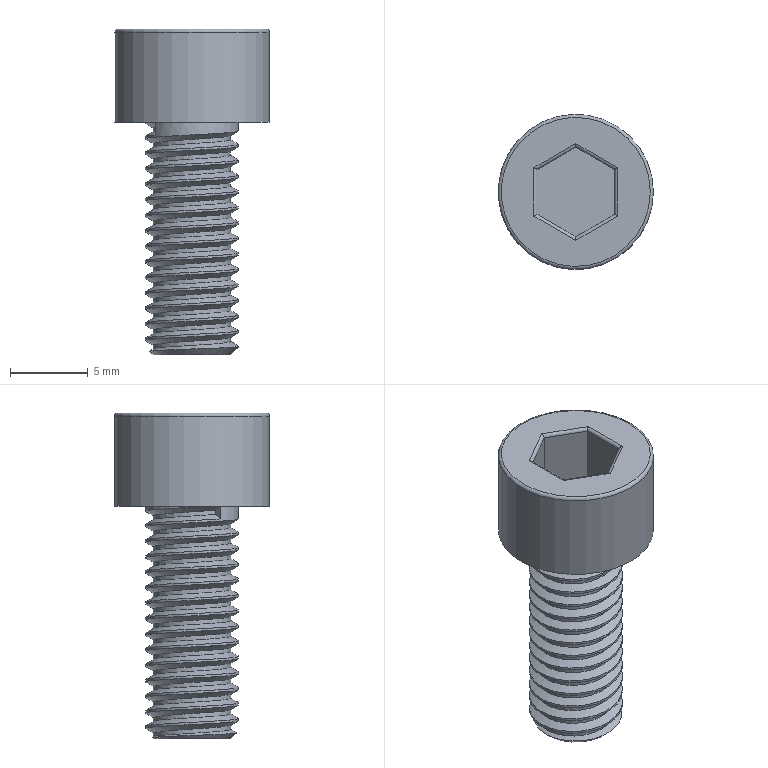Part | STEP file | Tube feed_id1098_x_t | 1 solid | 26 faces | box 10 x 10 x 21 mm | volume 739.091 mm3 | plane 12 | cylinder 9 | spline 3 | torus 1 | cone 1 | commonest cylinder face diameters 0.4 x6 5 x1 6 x1 10 x1